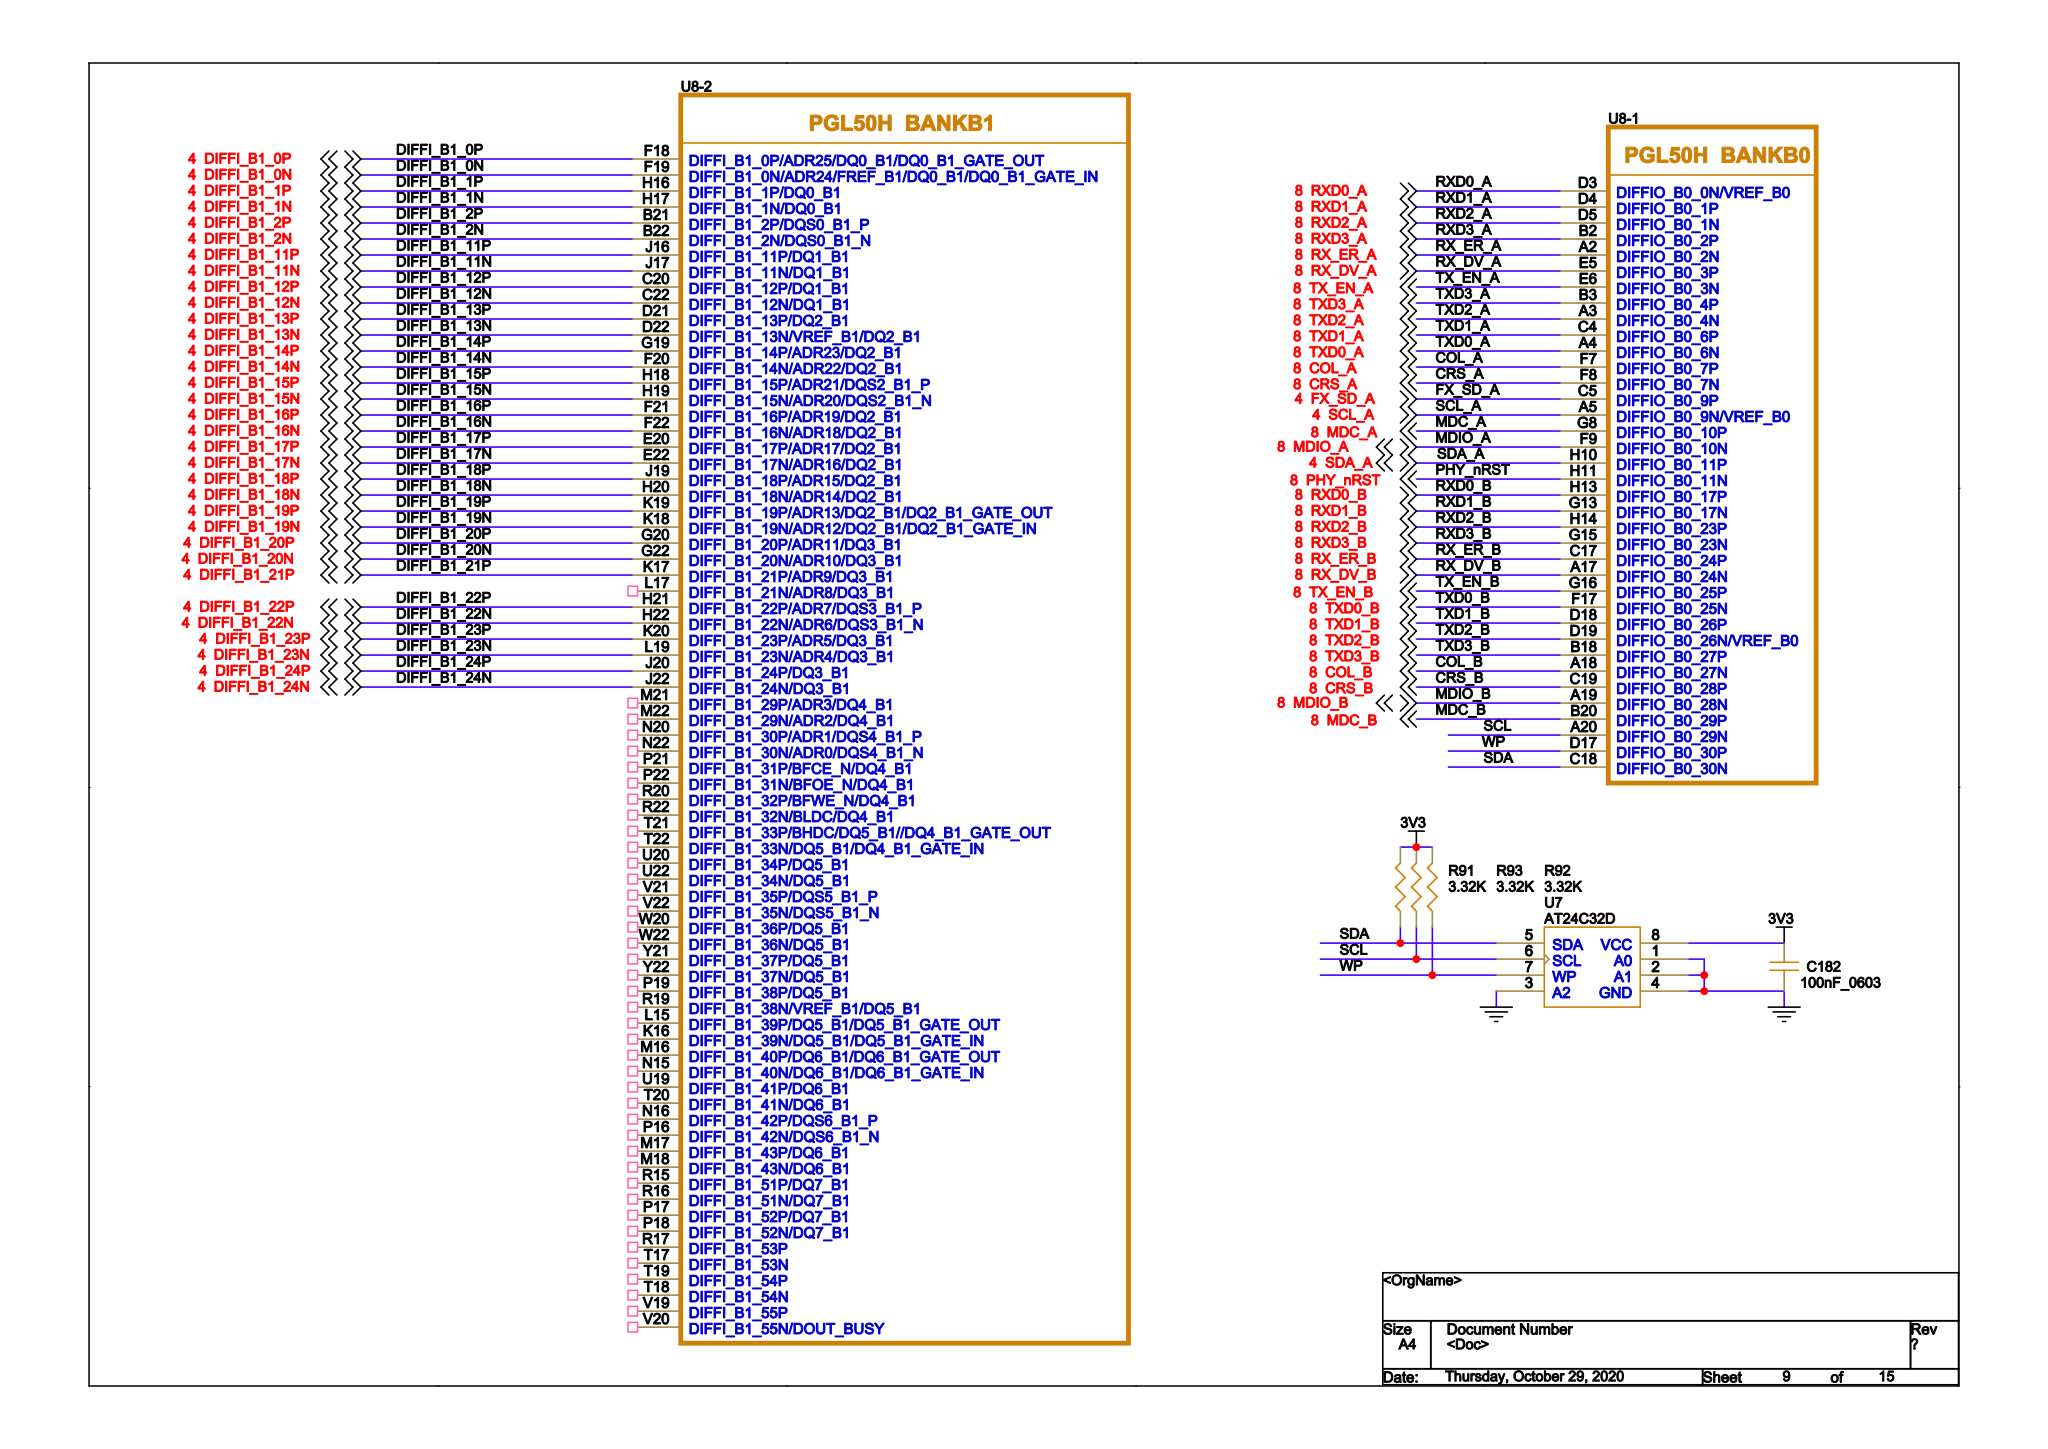Circuit board | Cadence Allegro | 406 parts | 392 nets | one sheet of the schematic
Parts on this sheet (reference | value | footprint):
C182 | 100nF_0603 | C_0603_104
R91 | 3.32K | R_0603
R92 | 3.32K | R_0603
R93 | 3.32K | R_0603
U7 | AT24C32D | U_SO8
Nets of these parts (net: part-pin ...):
GND: C182-2 U7-1 U7-2 U7-3 U7-4
3V3: C182-1 R91-2 R92-2 R93-2 U7-8
SDA: R91-1 U7-5
WP: R92-1 U7-7
SCL: R93-1 U7-6